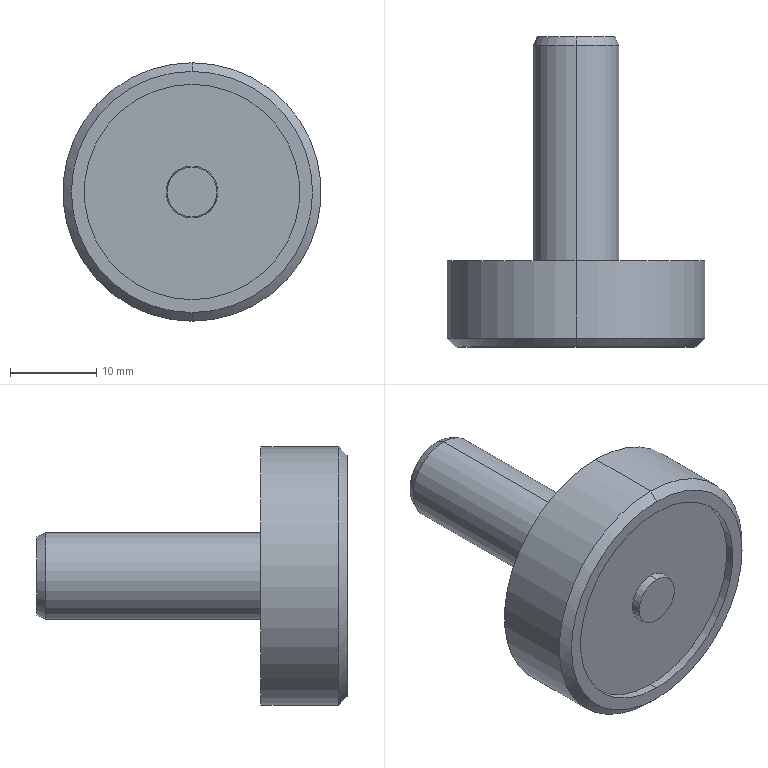Part | SolidWorks | features BaseBody 1 | 1 solid | 17 faces | box 30 x 36 x 30 mm | volume 8594 mm3 | cylinder 6 | cone 6 | plane 5 | commonest cylinder face diameters 10 x2 25 x2 30 x2
STEP:
#1=CARTESIAN_POINT('',(257.5,25.,218.121));
#2=VERTEX_POINT('',#1);
#3=CARTESIAN_POINT('',(257.5,25.,188.121));
#4=VERTEX_POINT('',#3);
#5=CARTESIAN_POINT('',(257.5,25.,203.121));
#6=DIRECTION('',(0.,1.,0.));
#7=DIRECTION('',(0.,0.,1.));
#8=AXIS2_PLACEMENT_3D('',#5,#6,#7);
#9=CIRCLE('',#8,15.);
#10=EDGE_CURVE('',#2,#4,#9,.T.);
#11=ORIENTED_EDGE('',*,*,#10,.T.);
#12=CARTESIAN_POINT('',(257.5,34.,188.121));
#13=VERTEX_POINT('',#12);
#14=CARTESIAN_POINT('',(257.5,60.,188.121));
#15=DIRECTION('',(0.,1.,0.));
#16=VECTOR('',#15,1000.);
#17=LINE('',#14,#16);
#18=EDGE_CURVE('',#4,#13,#17,.T.);
#19=ORIENTED_EDGE('',*,*,#18,.T.);
#20=CARTESIAN_POINT('',(257.5,34.,218.121));
#21=VERTEX_POINT('',#20);
#22=CARTESIAN_POINT('',(257.5,34.,203.121));
#23=DIRECTION('',(0.,1.,0.));
#24=DIRECTION('',(0.,0.,1.));
#25=AXIS2_PLACEMENT_3D('',#22,#23,#24);
#26=CIRCLE('',#25,15.);
#27=EDGE_CURVE('',#21,#13,#26,.T.);
#28=ORIENTED_EDGE('',*,*,#27,.F.);
#29=CARTESIAN_POINT('',(257.5,60.,218.121));
#30=DIRECTION('',(0.,1.,0.));
#31=VECTOR('',#30,1000.);
#32=LINE('',#29,#31);
#33=EDGE_CURVE('',#2,#21,#32,.T.);
#34=ORIENTED_EDGE('',*,*,#33,.F.);
#35=EDGE_LOOP('',(#11,#19,#28,#34));
#36=FACE_OUTER_BOUND('',#35,.T.);
#37=CARTESIAN_POINT('',(257.5,60.,203.121));
#38=DIRECTION('',(0.,1.,0.));
#39=DIRECTION('',(0.,0.,1.));
#40=AXIS2_PLACEMENT_3D('',#37,#38,#39);
#41=CYLINDRICAL_SURFACE('',#40,15.);
#42=ADVANCED_FACE('',(#36),#41,.T.);
#43=CARTESIAN_POINT('',(257.5,34.,198.121));
#44=VERTEX_POINT('',#43);
#45=CARTESIAN_POINT('',(257.5,34.,208.121));
#46=VERTEX_POINT('',#45);
#47=CARTESIAN_POINT('',(257.5,34.,203.121));
#48=DIRECTION('',(0.,-1.,0.));
#49=DIRECTION('',(0.,0.,1.));
#50=AXIS2_PLACEMENT_3D('',#47,#48,#49);
#51=CIRCLE('',#50,5.);
#52=EDGE_CURVE('',#44,#46,#51,.T.);
#53=ORIENTED_EDGE('',*,*,#52,.F.);
#54=CARTESIAN_POINT('',(257.5,59.,198.121));
#55=VERTEX_POINT('',#54);
#56=CARTESIAN_POINT('',(257.5,60.,198.121));
#57=DIRECTION('',(0.,1.,0.));
#58=VECTOR('',#57,1000.);
#59=LINE('',#56,#58);
#60=EDGE_CURVE('',#44,#55,#59,.T.);
#61=ORIENTED_EDGE('',*,*,#60,.T.);
#62=CARTESIAN_POINT('',(257.5,59.,208.121));
#63=VERTEX_POINT('',#62);
#64=CARTESIAN_POINT('',(257.5,59.,203.121));
#65=DIRECTION('',(0.,-1.,0.));
#66=DIRECTION('',(0.,0.,1.));
#67=AXIS2_PLACEMENT_3D('',#64,#65,#66);
#68=CIRCLE('',#67,5.);
#69=EDGE_CURVE('',#55,#63,#68,.T.);
#70=ORIENTED_EDGE('',*,*,#69,.T.);
#71=CARTESIAN_POINT('',(257.5,60.,208.121));
#72=DIRECTION('',(0.,1.,0.));
#73=VECTOR('',#72,1000.);
#74=LINE('',#71,#73);
#75=EDGE_CURVE('',#46,#63,#74,.T.);
#76=ORIENTED_EDGE('',*,*,#75,.F.);
#77=EDGE_LOOP('',(#53,#61,#70,#76));
#78=FACE_OUTER_BOUND('',#77,.T.);
#79=CARTESIAN_POINT('',(257.5,60.,203.121));
#80=DIRECTION('',(0.,1.,0.));
#81=DIRECTION('',(0.,0.,1.));
#82=AXIS2_PLACEMENT_3D('',#79,#80,#81);
#83=CYLINDRICAL_SURFACE('',#82,5.);
#84=ADVANCED_FACE('',(#78),#83,.T.);
#85=CARTESIAN_POINT('',(257.5,24.,217.121));
#86=VERTEX_POINT('',#85);
#87=CARTESIAN_POINT('',(257.5,24.,189.121));
#88=VERTEX_POINT('',#87);
#89=CARTESIAN_POINT('',(257.5,24.,203.121));
#90=DIRECTION('',(0.,1.,0.));
#91=DIRECTION('',(0.,0.,1.));
#92=AXIS2_PLACEMENT_3D('',#89,#90,#91);
#93=CIRCLE('',#92,14.);
#94=EDGE_CURVE('',#86,#88,#93,.T.);
#95=ORIENTED_EDGE('',*,*,#94,.T.);
#96=CARTESIAN_POINT('',(257.5,25.,188.121));
#97=DIRECTION('',(0.,0.7071,-0.7071));
#98=VECTOR('',#97,1000.);
#99=LINE('',#96,#98);
#100=EDGE_CURVE('',#88,#4,#99,.T.);
#101=ORIENTED_EDGE('',*,*,#100,.T.);
#102=ORIENTED_EDGE('',*,*,#10,.F.);
#103=CARTESIAN_POINT('',(257.5,25.,218.121));
#104=DIRECTION('',(0.,0.7071,0.7071));
#105=VECTOR('',#104,1000.);
#106=LINE('',#103,#105);
#107=EDGE_CURVE('',#86,#2,#106,.T.);
#108=ORIENTED_EDGE('',*,*,#107,.F.);
#109=EDGE_LOOP('',(#95,#101,#102,#108));
#110=FACE_OUTER_BOUND('',#109,.T.);
#111=CARTESIAN_POINT('',(257.5,25.,203.121));
#112=DIRECTION('',(0.,1.,0.));
#113=DIRECTION('',(0.,0.,1.));
#114=AXIS2_PLACEMENT_3D('',#111,#112,#113);
#115=CONICAL_SURFACE('',#114,15.,0.7854);
#116=ADVANCED_FACE('',(#110),#115,.T.);
#117=CARTESIAN_POINT('',(257.5,60.,198.587));
#118=VERTEX_POINT('',#117);
#119=CARTESIAN_POINT('',(257.5,60.,207.655));
#120=VERTEX_POINT('',#119);
#121=CARTESIAN_POINT('',(257.5,60.,203.121));
#122=DIRECTION('',(0.,-1.,0.));
#123=DIRECTION('',(0.,0.,-1.));
#124=AXIS2_PLACEMENT_3D('',#121,#122,#123);
#125=CIRCLE('',#124,4.534);
#126=EDGE_CURVE('',#118,#120,#125,.T.);
#127=ORIENTED_EDGE('',*,*,#126,.T.);
#128=CARTESIAN_POINT('',(257.5,59.,208.121));
#129=DIRECTION('',(0.,-0.9063,0.4226));
#130=VECTOR('',#129,1000.);
#131=LINE('',#128,#130);
#132=EDGE_CURVE('',#120,#63,#131,.T.);
#133=ORIENTED_EDGE('',*,*,#132,.T.);
#134=ORIENTED_EDGE('',*,*,#69,.F.);
#135=CARTESIAN_POINT('',(257.5,59.,198.121));
#136=DIRECTION('',(0.,-0.9063,-0.4226));
#137=VECTOR('',#136,1000.);
#138=LINE('',#135,#137);
#139=EDGE_CURVE('',#118,#55,#138,.T.);
#140=ORIENTED_EDGE('',*,*,#139,.F.);
#141=EDGE_LOOP('',(#127,#133,#134,#140));
#142=FACE_OUTER_BOUND('',#141,.T.);
#143=CARTESIAN_POINT('',(257.5,59.,203.121));
#144=DIRECTION('',(0.,-1.,0.));
#145=DIRECTION('',(0.,0.,-1.));
#146=AXIS2_PLACEMENT_3D('',#143,#144,#145);
#147=CONICAL_SURFACE('',#146,5.,0.4363);
#148=ADVANCED_FACE('',(#142),#147,.T.);
#149=CARTESIAN_POINT('',(257.5,25.,215.621));
#150=VERTEX_POINT('',#149);
#151=CARTESIAN_POINT('',(257.5,25.,190.621));
#152=VERTEX_POINT('',#151);
#153=CARTESIAN_POINT('',(257.5,25.,203.121));
#154=DIRECTION('',(0.,-1.,0.));
#155=DIRECTION('',(0.,0.,-1.));
#156=AXIS2_PLACEMENT_3D('',#153,#154,#155);
#157=CIRCLE('',#156,12.5);
#158=EDGE_CURVE('',#150,#152,#157,.T.);
#159=ORIENTED_EDGE('',*,*,#158,.F.);
#160=CARTESIAN_POINT('',(257.5,24.,215.621));
#161=VERTEX_POINT('',#160);
#162=CARTESIAN_POINT('',(257.5,25.,215.621));
#163=DIRECTION('',(0.,-1.,0.));
#164=VECTOR('',#163,1000.);
#165=LINE('',#162,#164);
#166=EDGE_CURVE('',#150,#161,#165,.T.);
#167=ORIENTED_EDGE('',*,*,#166,.T.);
#168=CARTESIAN_POINT('',(257.5,24.,190.621));
#169=VERTEX_POINT('',#168);
#170=CARTESIAN_POINT('',(257.5,24.,203.121));
#171=DIRECTION('',(0.,1.,0.));
#172=DIRECTION('',(0.,0.,-1.));
#173=AXIS2_PLACEMENT_3D('',#170,#171,#172);
#174=CIRCLE('',#173,12.5);
#175=EDGE_CURVE('',#169,#161,#174,.T.);
#176=ORIENTED_EDGE('',*,*,#175,.F.);
#177=CARTESIAN_POINT('',(257.5,25.,190.621));
#178=DIRECTION('',(0.,-1.,0.));
#179=VECTOR('',#178,1000.);
#180=LINE('',#177,#179);
#181=EDGE_CURVE('',#152,#169,#180,.T.);
#182=ORIENTED_EDGE('',*,*,#181,.F.);
#183=EDGE_LOOP('',(#159,#167,#176,#182));
#184=FACE_OUTER_BOUND('',#183,.T.);
#185=CARTESIAN_POINT('',(257.5,25.,203.121));
#186=DIRECTION('',(0.,-1.,0.));
#187=DIRECTION('',(0.,0.,-1.));
#188=AXIS2_PLACEMENT_3D('',#185,#186,#187);
#189=CYLINDRICAL_SURFACE('',#188,12.5);
#190=ADVANCED_FACE('',(#184),#189,.F.);
#191=CARTESIAN_POINT('',(257.5,24.,206.016));
#192=VERTEX_POINT('',#191);
#193=CARTESIAN_POINT('',(257.5,24.,200.226));
#194=VERTEX_POINT('',#193);
#195=CARTESIAN_POINT('',(257.5,24.,203.121));
#196=DIRECTION('',(0.,1.,0.));
#197=DIRECTION('',(0.,0.,1.));
#198=AXIS2_PLACEMENT_3D('',#195,#196,#197);
#199=CIRCLE('',#198,2.895);
#200=EDGE_CURVE('',#192,#194,#199,.T.);
#201=ORIENTED_EDGE('',*,*,#200,.T.);
#202=CARTESIAN_POINT('',(257.5,25.,200.121));
#203=VERTEX_POINT('',#202);
#204=CARTESIAN_POINT('',(257.5,25.,200.121));
#205=DIRECTION('',(0.,0.9945,-0.1045));
#206=VECTOR('',#205,1000.);
#207=LINE('',#204,#206);
#208=EDGE_CURVE('',#194,#203,#207,.T.);
#209=ORIENTED_EDGE('',*,*,#208,.T.);
#210=CARTESIAN_POINT('',(257.5,25.,206.121));
#211=VERTEX_POINT('',#210);
#212=CARTESIAN_POINT('',(257.5,25.,203.121));
#213=DIRECTION('',(0.,1.,0.));
#214=DIRECTION('',(0.,0.,1.));
#215=AXIS2_PLACEMENT_3D('',#212,#213,#214);
#216=CIRCLE('',#215,3.);
#217=EDGE_CURVE('',#211,#203,#216,.T.);
#218=ORIENTED_EDGE('',*,*,#217,.F.);
#219=CARTESIAN_POINT('',(257.5,25.,206.121));
#220=DIRECTION('',(0.,0.9945,0.1045));
#221=VECTOR('',#220,1000.);
#222=LINE('',#219,#221);
#223=EDGE_CURVE('',#192,#211,#222,.T.);
#224=ORIENTED_EDGE('',*,*,#223,.F.);
#225=EDGE_LOOP('',(#201,#209,#218,#224));
#226=FACE_OUTER_BOUND('',#225,.T.);
#227=CARTESIAN_POINT('',(257.5,25.,203.121));
#228=DIRECTION('',(0.,1.,0.));
#229=DIRECTION('',(0.,0.,1.));
#230=AXIS2_PLACEMENT_3D('',#227,#228,#229);
#231=CONICAL_SURFACE('',#230,3.,0.1047);
#232=ADVANCED_FACE('',(#226),#231,.T.);
#233=ORIENTED_EDGE('',*,*,#27,.T.);
#234=CARTESIAN_POINT('',(257.5,34.,203.121));
#235=DIRECTION('',(0.,1.,0.));
#236=DIRECTION('',(0.,0.,1.));
#237=AXIS2_PLACEMENT_3D('',#234,#235,#236);
#238=CIRCLE('',#237,15.);
#239=EDGE_CURVE('',#13,#21,#238,.T.);
#240=ORIENTED_EDGE('',*,*,#239,.T.);
#241=EDGE_LOOP('',(#233,#240));
#242=FACE_OUTER_BOUND('',#241,.T.);
#243=CARTESIAN_POINT('',(257.5,34.,203.121));
#244=DIRECTION('',(0.,-1.,0.));
#245=DIRECTION('',(0.,0.,1.));
#246=AXIS2_PLACEMENT_3D('',#243,#244,#245);
#247=CIRCLE('',#246,5.);
#248=EDGE_CURVE('',#46,#44,#247,.T.);
#249=ORIENTED_EDGE('',*,*,#248,.T.);
#250=ORIENTED_EDGE('',*,*,#52,.T.);
#251=EDGE_LOOP('',(#249,#250));
#252=FACE_BOUND('',#251,.T.);
#253=CARTESIAN_POINT('',(242.892,34.,206.527));
#254=DIRECTION('',(0.,1.,0.));
#255=DIRECTION('',(0.,0.,1.));
#256=AXIS2_PLACEMENT_3D('',#253,#254,#255);
#257=PLANE('',#256);
#258=ADVANCED_FACE('',(#242,#252),#257,.T.);
#259=ORIENTED_EDGE('',*,*,#18,.F.);
#260=CARTESIAN_POINT('',(257.5,25.,203.121));
#261=DIRECTION('',(0.,1.,0.));
#262=DIRECTION('',(0.,0.,1.));
#263=AXIS2_PLACEMENT_3D('',#260,#261,#262);
#264=CIRCLE('',#263,15.);
#265=EDGE_CURVE('',#4,#2,#264,.T.);
#266=ORIENTED_EDGE('',*,*,#265,.T.);
#267=ORIENTED_EDGE('',*,*,#33,.T.);
#268=ORIENTED_EDGE('',*,*,#239,.F.);
#269=EDGE_LOOP('',(#259,#266,#267,#268));
#270=FACE_OUTER_BOUND('',#269,.T.);
#271=CARTESIAN_POINT('',(257.5,60.,203.121));
#272=DIRECTION('',(0.,1.,0.));
#273=DIRECTION('',(0.,0.,1.));
#274=AXIS2_PLACEMENT_3D('',#271,#272,#273);
#275=CYLINDRICAL_SURFACE('',#274,15.);
#276=ADVANCED_FACE('',(#270),#275,.T.);
#277=ORIENTED_EDGE('',*,*,#60,.F.);
#278=ORIENTED_EDGE('',*,*,#248,.F.);
#279=ORIENTED_EDGE('',*,*,#75,.T.);
#280=CARTESIAN_POINT('',(257.5,59.,203.121));
#281=DIRECTION('',(0.,-1.,0.));
#282=DIRECTION('',(0.,0.,1.));
#283=AXIS2_PLACEMENT_3D('',#280,#281,#282);
#284=CIRCLE('',#283,5.);
#285=EDGE_CURVE('',#63,#55,#284,.T.);
#286=ORIENTED_EDGE('',*,*,#285,.T.);
#287=EDGE_LOOP('',(#277,#278,#279,#286));
#288=FACE_OUTER_BOUND('',#287,.T.);
#289=CARTESIAN_POINT('',(257.5,60.,203.121));
#290=DIRECTION('',(0.,1.,0.));
#291=DIRECTION('',(0.,0.,1.));
#292=AXIS2_PLACEMENT_3D('',#289,#290,#291);
#293=CYLINDRICAL_SURFACE('',#292,5.);
#294=ADVANCED_FACE('',(#288),#293,.T.);
#295=ORIENTED_EDGE('',*,*,#100,.F.);
#296=CARTESIAN_POINT('',(257.5,24.,203.121));
#297=DIRECTION('',(0.,1.,0.));
#298=DIRECTION('',(0.,0.,1.));
#299=AXIS2_PLACEMENT_3D('',#296,#297,#298);
#300=CIRCLE('',#299,14.);
#301=EDGE_CURVE('',#88,#86,#300,.T.);
#302=ORIENTED_EDGE('',*,*,#301,.T.);
#303=ORIENTED_EDGE('',*,*,#107,.T.);
#304=ORIENTED_EDGE('',*,*,#265,.F.);
#305=EDGE_LOOP('',(#295,#302,#303,#304));
#306=FACE_OUTER_BOUND('',#305,.T.);
#307=CARTESIAN_POINT('',(257.5,25.,203.121));
#308=DIRECTION('',(0.,1.,0.));
#309=DIRECTION('',(0.,0.,1.));
#310=AXIS2_PLACEMENT_3D('',#307,#308,#309);
#311=CONICAL_SURFACE('',#310,15.,0.7854);
#312=ADVANCED_FACE('',(#306),#311,.T.);
#313=ORIENTED_EDGE('',*,*,#132,.F.);
#314=CARTESIAN_POINT('',(257.5,60.,203.121));
#315=DIRECTION('',(0.,-1.,0.));
#316=DIRECTION('',(0.,0.,-1.));
#317=AXIS2_PLACEMENT_3D('',#314,#315,#316);
#318=CIRCLE('',#317,4.534);
#319=EDGE_CURVE('',#120,#118,#318,.T.);
#320=ORIENTED_EDGE('',*,*,#319,.T.);
#321=ORIENTED_EDGE('',*,*,#139,.T.);
#322=ORIENTED_EDGE('',*,*,#285,.F.);
#323=EDGE_LOOP('',(#313,#320,#321,#322));
#324=FACE_OUTER_BOUND('',#323,.T.);
#325=CARTESIAN_POINT('',(257.5,59.,203.121));
#326=DIRECTION('',(0.,-1.,0.));
#327=DIRECTION('',(0.,0.,-1.));
#328=AXIS2_PLACEMENT_3D('',#325,#326,#327);
#329=CONICAL_SURFACE('',#328,5.,0.4363);
#330=ADVANCED_FACE('',(#324),#329,.T.);
#331=ORIENTED_EDGE('',*,*,#94,.F.);
#332=ORIENTED_EDGE('',*,*,#301,.F.);
#333=EDGE_LOOP('',(#331,#332));
#334=FACE_OUTER_BOUND('',#333,.T.);
#335=ORIENTED_EDGE('',*,*,#175,.T.);
#336=CARTESIAN_POINT('',(257.5,24.,203.121));
#337=DIRECTION('',(0.,1.,0.));
#338=DIRECTION('',(0.,0.,-1.));
#339=AXIS2_PLACEMENT_3D('',#336,#337,#338);
#340=CIRCLE('',#339,12.5);
#341=EDGE_CURVE('',#161,#169,#340,.T.);
#342=ORIENTED_EDGE('',*,*,#341,.T.);
#343=EDGE_LOOP('',(#335,#342));
#344=FACE_BOUND('',#343,.T.);
#345=CARTESIAN_POINT('',(257.5,24.,203.121));
#346=DIRECTION('',(0.,-1.,0.));
#347=DIRECTION('',(0.,0.,-1.));
#348=AXIS2_PLACEMENT_3D('',#345,#346,#347);
#349=PLANE('',#348);
#350=ADVANCED_FACE('',(#334,#344),#349,.T.);
#351=ORIENTED_EDGE('',*,*,#126,.F.);
#352=ORIENTED_EDGE('',*,*,#319,.F.);
#353=EDGE_LOOP('',(#351,#352));
#354=FACE_OUTER_BOUND('',#353,.T.);
#355=CARTESIAN_POINT('',(252.631,60.,204.256));
#356=DIRECTION('',(0.,1.,0.));
#357=DIRECTION('',(0.,0.,1.));
#358=AXIS2_PLACEMENT_3D('',#355,#356,#357);
#359=PLANE('',#358);
#360=ADVANCED_FACE('',(#354),#359,.T.);
#361=ORIENTED_EDGE('',*,*,#166,.F.);
#362=CARTESIAN_POINT('',(257.5,25.,203.121));
#363=DIRECTION('',(0.,-1.,0.));
#364=DIRECTION('',(0.,0.,-1.));
#365=AXIS2_PLACEMENT_3D('',#362,#363,#364);
#366=CIRCLE('',#365,12.5);
#367=EDGE_CURVE('',#152,#150,#366,.T.);
#368=ORIENTED_EDGE('',*,*,#367,.F.);
#369=ORIENTED_EDGE('',*,*,#181,.T.);
#370=ORIENTED_EDGE('',*,*,#341,.F.);
#371=EDGE_LOOP('',(#361,#368,#369,#370));
#372=FACE_OUTER_BOUND('',#371,.T.);
#373=CARTESIAN_POINT('',(257.5,25.,203.121));
#374=DIRECTION('',(0.,-1.,0.));
#375=DIRECTION('',(0.,0.,-1.));
#376=AXIS2_PLACEMENT_3D('',#373,#374,#375);
#377=CYLINDRICAL_SURFACE('',#376,12.5);
#378=ADVANCED_FACE('',(#372),#377,.F.);
#379=ORIENTED_EDGE('',*,*,#217,.T.);
#380=CARTESIAN_POINT('',(257.5,25.,203.121));
#381=DIRECTION('',(0.,1.,0.));
#382=DIRECTION('',(0.,0.,1.));
#383=AXIS2_PLACEMENT_3D('',#380,#381,#382);
#384=CIRCLE('',#383,3.);
#385=EDGE_CURVE('',#203,#211,#384,.T.);
#386=ORIENTED_EDGE('',*,*,#385,.T.);
#387=EDGE_LOOP('',(#379,#386));
#388=FACE_BOUND('',#387,.T.);
#389=ORIENTED_EDGE('',*,*,#367,.T.);
#390=ORIENTED_EDGE('',*,*,#158,.T.);
#391=EDGE_LOOP('',(#389,#390));
#392=FACE_OUTER_BOUND('',#391,.T.);
#393=CARTESIAN_POINT('',(257.5,25.,203.121));
#394=DIRECTION('',(0.,-1.,0.));
#395=DIRECTION('',(0.,0.,-1.));
#396=AXIS2_PLACEMENT_3D('',#393,#394,#395);
#397=PLANE('',#396);
#398=ADVANCED_FACE('',(#388,#392),#397,.T.);
#399=ORIENTED_EDGE('',*,*,#208,.F.);
#400=CARTESIAN_POINT('',(257.5,24.,203.121));
#401=DIRECTION('',(0.,1.,0.));
#402=DIRECTION('',(0.,0.,1.));
#403=AXIS2_PLACEMENT_3D('',#400,#401,#402);
#404=CIRCLE('',#403,2.895);
#405=EDGE_CURVE('',#194,#192,#404,.T.);
#406=ORIENTED_EDGE('',*,*,#405,.T.);
#407=ORIENTED_EDGE('',*,*,#223,.T.);
#408=ORIENTED_EDGE('',*,*,#385,.F.);
#409=EDGE_LOOP('',(#399,#406,#407,#408));
#410=FACE_OUTER_BOUND('',#409,.T.);
#411=CARTESIAN_POINT('',(257.5,25.,203.121));
#412=DIRECTION('',(0.,1.,0.));
#413=DIRECTION('',(0.,0.,1.));
#414=AXIS2_PLACEMENT_3D('',#411,#412,#413);
#415=CONICAL_SURFACE('',#414,3.,0.1047);
#416=ADVANCED_FACE('',(#410),#415,.T.);
#417=ORIENTED_EDGE('',*,*,#200,.F.);
#418=ORIENTED_EDGE('',*,*,#405,.F.);
#419=EDGE_LOOP('',(#417,#418));
#420=FACE_OUTER_BOUND('',#419,.T.);
#421=CARTESIAN_POINT('',(257.5,24.,203.121));
#422=DIRECTION('',(0.,-1.,0.));
#423=DIRECTION('',(0.,0.,-1.));
#424=AXIS2_PLACEMENT_3D('',#421,#422,#423);
#425=PLANE('',#424);
#426=ADVANCED_FACE('',(#420),#425,.T.);
#427=CLOSED_SHELL('',(#42,#84,#116,#148,#190,#232,#258,#276,#294,#312,#330,#350,#360,#378,#398,#416,#426));
#428=MANIFOLD_SOLID_BREP('',#427);
#429=CARTESIAN_POINT('',(0.,0.,0.));
#430=DIRECTION('',(0.,0.,1.));
#431=DIRECTION('',(1.,0.,0.));
#432=AXIS2_PLACEMENT_3D('',#429,#430,#431);
#433=(LENGTH_UNIT()NAMED_UNIT(*)SI_UNIT(.MILLI.,.METRE.));
#434=UNCERTAINTY_MEASURE_WITH_UNIT(LENGTH_MEASURE(0.00001),#433,'','');
#435=(NAMED_UNIT(*)PLANE_ANGLE_UNIT()SI_UNIT($,.RADIAN.));
#436=(NAMED_UNIT(*)SI_UNIT($,.STERADIAN.)SOLID_ANGLE_UNIT());
#437=(GEOMETRIC_REPRESENTATION_CONTEXT(3)GLOBAL_UNCERTAINTY_ASSIGNED_CONTEXT((#434))GLOBAL_UNIT_ASSIGNED_CONTEXT((#433,#435,#436))REPRESENTATION_CONTEXT('',''));
#438=ADVANCED_BREP_SHAPE_REPRESENTATION('',(#428,#432),#437);